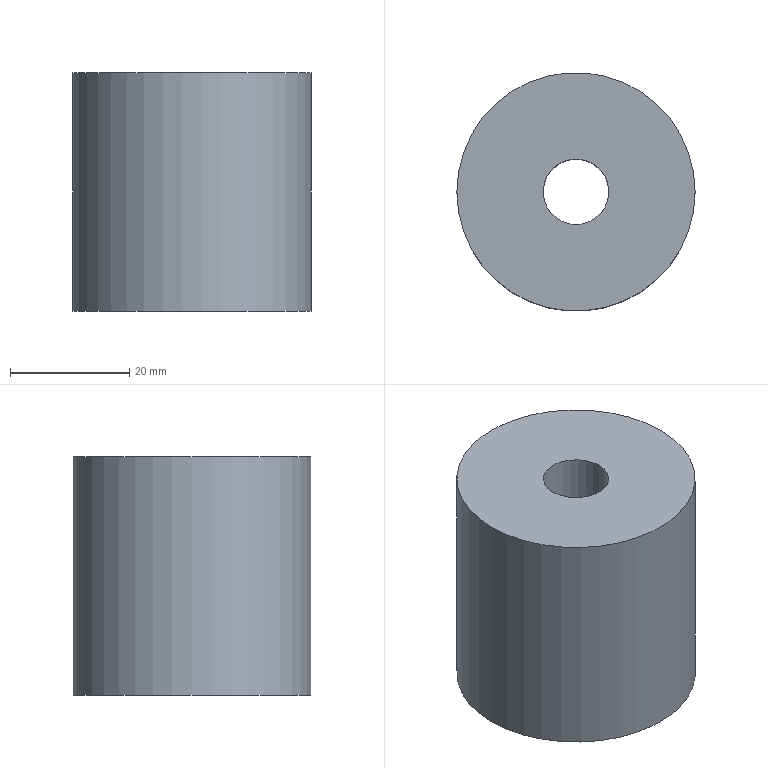Part | STEP file | PN_0009_id1210_x_t | 1 solid | 6 faces | box 40 x 40 x 40 mm | volume 44485 mm3 | plane 3 | cylinder 3 | commonest cylinder face diameters 11 x1 17 x1 40 x1
STEP:
#1=CARTESIAN_POINT('',(-285.,-92.5,65.));
#2=VERTEX_POINT('',#1);
#3=CARTESIAN_POINT('',(-265.,-92.5,65.));
#4=DIRECTION('',(0.,0.,1.));
#5=DIRECTION('',(-1.,0.,0.));
#6=AXIS2_PLACEMENT_3D('',#3,#4,#5);
#7=CIRCLE('',#6,20.);
#8=EDGE_CURVE('',#2,#2,#7,.T.);
#9=ORIENTED_EDGE('',*,*,#8,.F.);
#10=EDGE_LOOP('',(#9));
#11=FACE_BOUND('',#10,.T.);
#12=CARTESIAN_POINT('',(-273.5,-92.5,65.));
#13=VERTEX_POINT('',#12);
#14=CARTESIAN_POINT('',(-265.,-92.5,65.));
#15=DIRECTION('',(0.,0.,1.));
#16=DIRECTION('',(-1.,0.,0.));
#17=AXIS2_PLACEMENT_3D('',#14,#15,#16);
#18=CIRCLE('',#17,8.5);
#19=EDGE_CURVE('',#13,#13,#18,.T.);
#20=ORIENTED_EDGE('',*,*,#19,.T.);
#21=EDGE_LOOP('',(#20));
#22=FACE_BOUND('',#21,.T.);
#23=CARTESIAN_POINT('',(-265.,-92.5,65.));
#24=DIRECTION('',(0.,0.,-1.));
#25=DIRECTION('',(-1.,0.,0.));
#26=AXIS2_PLACEMENT_3D('',#23,#24,#25);
#27=PLANE('',#26);
#28=ADVANCED_FACE('',(#11,#22),#27,.T.);
#29=CARTESIAN_POINT('',(-285.,-92.5,105.));
#30=VERTEX_POINT('',#29);
#31=CARTESIAN_POINT('',(-265.,-92.5,105.));
#32=DIRECTION('',(0.,0.,-1.));
#33=DIRECTION('',(-1.,0.,0.));
#34=AXIS2_PLACEMENT_3D('',#31,#32,#33);
#35=CIRCLE('',#34,20.);
#36=EDGE_CURVE('',#30,#30,#35,.T.);
#37=ORIENTED_EDGE('',*,*,#36,.F.);
#38=EDGE_LOOP('',(#37));
#39=FACE_BOUND('',#38,.T.);
#40=CARTESIAN_POINT('',(-270.5,-92.5,105.));
#41=VERTEX_POINT('',#40);
#42=CARTESIAN_POINT('',(-265.,-92.5,105.));
#43=DIRECTION('',(0.,0.,-1.));
#44=DIRECTION('',(-1.,0.,0.));
#45=AXIS2_PLACEMENT_3D('',#42,#43,#44);
#46=CIRCLE('',#45,5.5);
#47=EDGE_CURVE('',#41,#41,#46,.T.);
#48=ORIENTED_EDGE('',*,*,#47,.T.);
#49=EDGE_LOOP('',(#48));
#50=FACE_BOUND('',#49,.T.);
#51=CARTESIAN_POINT('',(-265.,-92.5,105.));
#52=DIRECTION('',(0.,0.,1.));
#53=DIRECTION('',(1.,0.,0.));
#54=AXIS2_PLACEMENT_3D('',#51,#52,#53);
#55=PLANE('',#54);
#56=ADVANCED_FACE('',(#39,#50),#55,.T.);
#57=ORIENTED_EDGE('',*,*,#8,.T.);
#58=EDGE_LOOP('',(#57));
#59=FACE_BOUND('',#58,.T.);
#60=ORIENTED_EDGE('',*,*,#36,.T.);
#61=EDGE_LOOP('',(#60));
#62=FACE_BOUND('',#61,.T.);
#63=CARTESIAN_POINT('',(-265.,-92.5,105.));
#64=DIRECTION('',(0.,0.,-1.));
#65=DIRECTION('',(-1.,0.,0.));
#66=AXIS2_PLACEMENT_3D('',#63,#64,#65);
#67=CYLINDRICAL_SURFACE('',#66,20.);
#68=ADVANCED_FACE('',(#59,#62),#67,.T.);
#69=CARTESIAN_POINT('',(-259.5,-92.5,80.));
#70=VERTEX_POINT('',#69);
#71=CARTESIAN_POINT('',(-265.,-92.5,80.));
#72=DIRECTION('',(0.,0.,1.));
#73=DIRECTION('',(1.,0.,0.));
#74=AXIS2_PLACEMENT_3D('',#71,#72,#73);
#75=CIRCLE('',#74,5.5);
#76=EDGE_CURVE('',#70,#70,#75,.T.);
#77=ORIENTED_EDGE('',*,*,#76,.F.);
#78=EDGE_LOOP('',(#77));
#79=FACE_BOUND('',#78,.T.);
#80=ORIENTED_EDGE('',*,*,#47,.F.);
#81=EDGE_LOOP('',(#80));
#82=FACE_BOUND('',#81,.T.);
#83=CARTESIAN_POINT('',(-265.,-92.5,105.));
#84=DIRECTION('',(0.,0.,-1.));
#85=DIRECTION('',(-1.,0.,0.));
#86=AXIS2_PLACEMENT_3D('',#83,#84,#85);
#87=CYLINDRICAL_SURFACE('',#86,5.5);
#88=ADVANCED_FACE('',(#79,#82),#87,.F.);
#89=ORIENTED_EDGE('',*,*,#76,.T.);
#90=EDGE_LOOP('',(#89));
#91=FACE_BOUND('',#90,.T.);
#92=CARTESIAN_POINT('',(-273.5,-92.5,80.));
#93=VERTEX_POINT('',#92);
#94=CARTESIAN_POINT('',(-265.,-92.5,80.));
#95=DIRECTION('',(0.,0.,1.));
#96=DIRECTION('',(-1.,0.,0.));
#97=AXIS2_PLACEMENT_3D('',#94,#95,#96);
#98=CIRCLE('',#97,8.5);
#99=EDGE_CURVE('',#93,#93,#98,.T.);
#100=ORIENTED_EDGE('',*,*,#99,.F.);
#101=EDGE_LOOP('',(#100));
#102=FACE_BOUND('',#101,.T.);
#103=CARTESIAN_POINT('',(-265.,-92.5,80.));
#104=DIRECTION('',(0.,0.,1.));
#105=DIRECTION('',(1.,0.,0.));
#106=AXIS2_PLACEMENT_3D('',#103,#104,#105);
#107=PLANE('',#106);
#108=ADVANCED_FACE('',(#91,#102),#107,.F.);
#109=ORIENTED_EDGE('',*,*,#19,.F.);
#110=EDGE_LOOP('',(#109));
#111=FACE_BOUND('',#110,.T.);
#112=ORIENTED_EDGE('',*,*,#99,.T.);
#113=EDGE_LOOP('',(#112));
#114=FACE_BOUND('',#113,.T.);
#115=CARTESIAN_POINT('',(-265.,-92.5,80.));
#116=DIRECTION('',(0.,0.,-1.));
#117=DIRECTION('',(-1.,0.,0.));
#118=AXIS2_PLACEMENT_3D('',#115,#116,#117);
#119=CYLINDRICAL_SURFACE('',#118,8.5);
#120=ADVANCED_FACE('',(#111,#114),#119,.F.);
#121=CLOSED_SHELL('',(#28,#56,#68,#88,#108,#120));
#122=MANIFOLD_SOLID_BREP('',#121);
#123=(LENGTH_UNIT()NAMED_UNIT(*)SI_UNIT(.MILLI.,.METRE.));
#124=UNCERTAINTY_MEASURE_WITH_UNIT(LENGTH_MEASURE(0.00002),#123,'','');
#125=(NAMED_UNIT(*)PLANE_ANGLE_UNIT()SI_UNIT($,.RADIAN.));
#126=PLANE_ANGLE_MEASURE_WITH_UNIT(PLANE_ANGLE_MEASURE(0.01745),#125);
#127=DIMENSIONAL_EXPONENTS(0.,0.,0.,0.,0.,0.,0.);
#128=(CONVERSION_BASED_UNIT('DEGREE',#126)NAMED_UNIT(#127)PLANE_ANGLE_UNIT());
#129=(NAMED_UNIT(*)SI_UNIT($,.STERADIAN.)SOLID_ANGLE_UNIT());
#130=(GEOMETRIC_REPRESENTATION_CONTEXT(3)GLOBAL_UNCERTAINTY_ASSIGNED_CONTEXT((#124))GLOBAL_UNIT_ASSIGNED_CONTEXT((#123,#128,#129))REPRESENTATION_CONTEXT('',''));
#131=ADVANCED_BREP_SHAPE_REPRESENTATION('',(#122),#130);